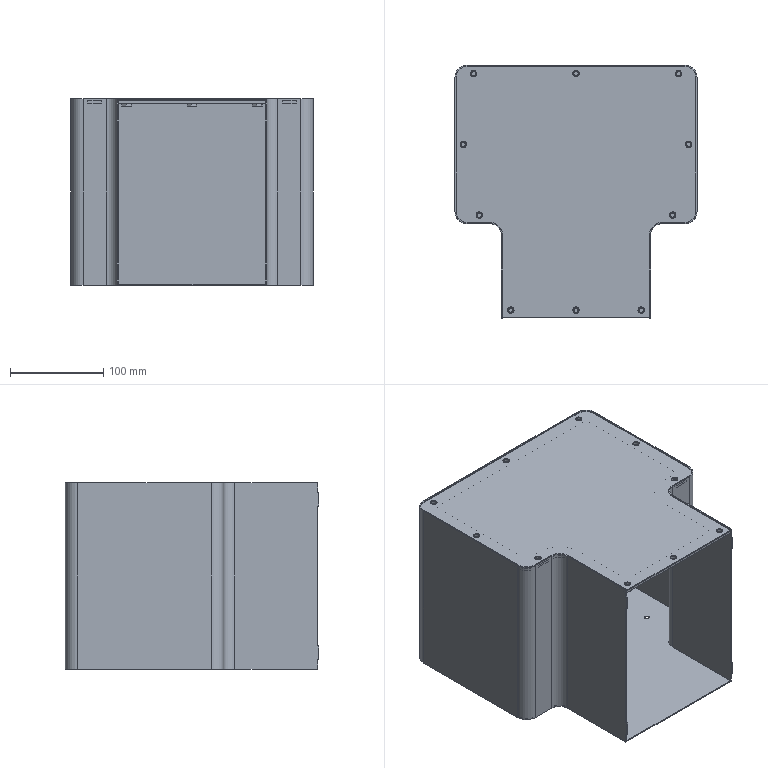Part | SolidWorks | 14 solids | 490 faces | box 260 x 272 x 200 mm | volume 384114 mm3 | plane 272 | cylinder 158 | cone 60 | commonest cylinder face diameters 7 x40 4.459 x20 6.96 x20 7.22 x20 24 x18 5 x16